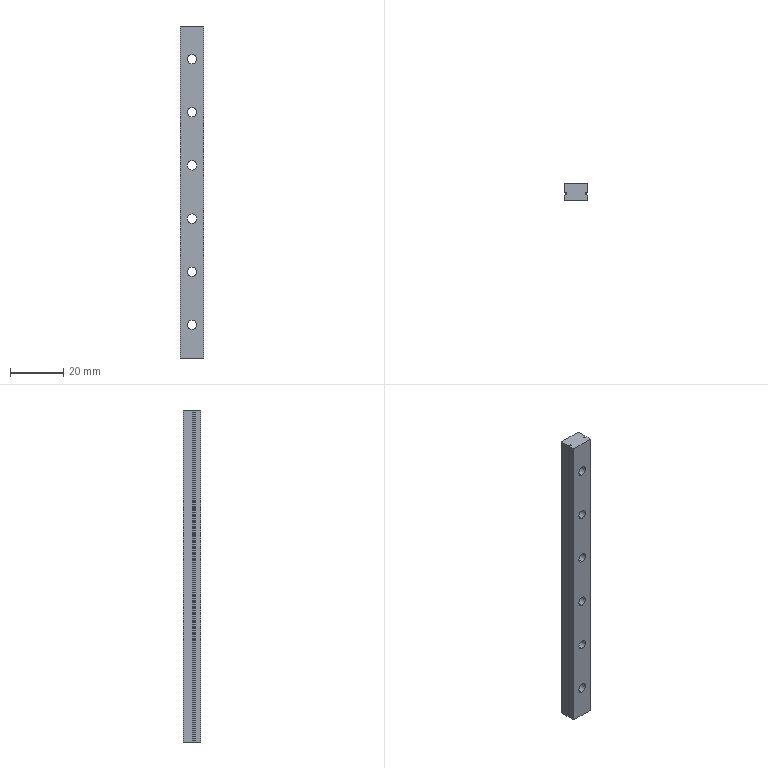Part | SolidWorks | features BaseBody 1 | 1 solid | 44 faces | box 9 x 6.5 x 125 mm | volume 6242 mm3 | cylinder 24 | plane 20 | commonest cylinder face diameters 3.5 x12 6.5 x12
STEP:
#1=CARTESIAN_POINT('',(0.,-3.25,249.25));
#2=VERTEX_POINT('',#1);
#3=CARTESIAN_POINT('',(0.,-3.25,245.75));
#4=VERTEX_POINT('',#3);
#5=CARTESIAN_POINT('',(0.,-3.25,247.5));
#6=DIRECTION('',(0.,-1.,0.));
#7=DIRECTION('',(0.,0.,1.));
#8=AXIS2_PLACEMENT_3D('',#5,#6,#7);
#9=CIRCLE('',#8,1.75);
#10=EDGE_CURVE('',#2,#4,#9,.T.);
#11=ORIENTED_EDGE('',*,*,#10,.T.);
#12=CARTESIAN_POINT('',(0.,-0.25,245.75));
#13=VERTEX_POINT('',#12);
#14=CARTESIAN_POINT('',(0.,-3.25,245.75));
#15=DIRECTION('',(0.,1.,0.));
#16=VECTOR('',#15,1000.);
#17=LINE('',#14,#16);
#18=EDGE_CURVE('',#4,#13,#17,.T.);
#19=ORIENTED_EDGE('',*,*,#18,.T.);
#20=CARTESIAN_POINT('',(0.,-0.25,249.25));
#21=VERTEX_POINT('',#20);
#22=CARTESIAN_POINT('',(0.,-0.25,247.5));
#23=DIRECTION('',(0.,-1.,0.));
#24=DIRECTION('',(0.,0.,1.));
#25=AXIS2_PLACEMENT_3D('',#22,#23,#24);
#26=CIRCLE('',#25,1.75);
#27=EDGE_CURVE('',#21,#13,#26,.T.);
#28=ORIENTED_EDGE('',*,*,#27,.F.);
#29=CARTESIAN_POINT('',(0.,-3.25,249.25));
#30=DIRECTION('',(0.,1.,0.));
#31=VECTOR('',#30,1000.);
#32=LINE('',#29,#31);
#33=EDGE_CURVE('',#2,#21,#32,.T.);
#34=ORIENTED_EDGE('',*,*,#33,.F.);
#35=EDGE_LOOP('',(#11,#19,#28,#34));
#36=FACE_OUTER_BOUND('',#35,.T.);
#37=CARTESIAN_POINT('',(0.,-3.25,247.5));
#38=DIRECTION('',(0.,1.,0.));
#39=DIRECTION('',(0.,0.,1.));
#40=AXIS2_PLACEMENT_3D('',#37,#38,#39);
#41=CYLINDRICAL_SURFACE('',#40,1.75);
#42=ADVANCED_FACE('',(#36),#41,.F.);
#43=CARTESIAN_POINT('',(0.,-3.25,229.25));
#44=VERTEX_POINT('',#43);
#45=CARTESIAN_POINT('',(0.,-3.25,225.75));
#46=VERTEX_POINT('',#45);
#47=CARTESIAN_POINT('',(0.,-3.25,227.5));
#48=DIRECTION('',(0.,-1.,0.));
#49=DIRECTION('',(0.,0.,1.));
#50=AXIS2_PLACEMENT_3D('',#47,#48,#49);
#51=CIRCLE('',#50,1.75);
#52=EDGE_CURVE('',#44,#46,#51,.T.);
#53=ORIENTED_EDGE('',*,*,#52,.T.);
#54=CARTESIAN_POINT('',(0.,-0.25,225.75));
#55=VERTEX_POINT('',#54);
#56=CARTESIAN_POINT('',(0.,-3.25,225.75));
#57=DIRECTION('',(0.,1.,0.));
#58=VECTOR('',#57,1000.);
#59=LINE('',#56,#58);
#60=EDGE_CURVE('',#46,#55,#59,.T.);
#61=ORIENTED_EDGE('',*,*,#60,.T.);
#62=CARTESIAN_POINT('',(0.,-0.25,229.25));
#63=VERTEX_POINT('',#62);
#64=CARTESIAN_POINT('',(0.,-0.25,227.5));
#65=DIRECTION('',(0.,-1.,0.));
#66=DIRECTION('',(0.,0.,1.));
#67=AXIS2_PLACEMENT_3D('',#64,#65,#66);
#68=CIRCLE('',#67,1.75);
#69=EDGE_CURVE('',#63,#55,#68,.T.);
#70=ORIENTED_EDGE('',*,*,#69,.F.);
#71=CARTESIAN_POINT('',(0.,-3.25,229.25));
#72=DIRECTION('',(0.,1.,0.));
#73=VECTOR('',#72,1000.);
#74=LINE('',#71,#73);
#75=EDGE_CURVE('',#44,#63,#74,.T.);
#76=ORIENTED_EDGE('',*,*,#75,.F.);
#77=EDGE_LOOP('',(#53,#61,#70,#76));
#78=FACE_OUTER_BOUND('',#77,.T.);
#79=CARTESIAN_POINT('',(0.,-3.25,227.5));
#80=DIRECTION('',(0.,1.,0.));
#81=DIRECTION('',(0.,0.,1.));
#82=AXIS2_PLACEMENT_3D('',#79,#80,#81);
#83=CYLINDRICAL_SURFACE('',#82,1.75);
#84=ADVANCED_FACE('',(#78),#83,.F.);
#85=CARTESIAN_POINT('',(0.,-3.25,209.25));
#86=VERTEX_POINT('',#85);
#87=CARTESIAN_POINT('',(0.,-3.25,205.75));
#88=VERTEX_POINT('',#87);
#89=CARTESIAN_POINT('',(0.,-3.25,207.5));
#90=DIRECTION('',(0.,-1.,0.));
#91=DIRECTION('',(0.,0.,1.));
#92=AXIS2_PLACEMENT_3D('',#89,#90,#91);
#93=CIRCLE('',#92,1.75);
#94=EDGE_CURVE('',#86,#88,#93,.T.);
#95=ORIENTED_EDGE('',*,*,#94,.T.);
#96=CARTESIAN_POINT('',(0.,-0.25,205.75));
#97=VERTEX_POINT('',#96);
#98=CARTESIAN_POINT('',(0.,-3.25,205.75));
#99=DIRECTION('',(0.,1.,0.));
#100=VECTOR('',#99,1000.);
#101=LINE('',#98,#100);
#102=EDGE_CURVE('',#88,#97,#101,.T.);
#103=ORIENTED_EDGE('',*,*,#102,.T.);
#104=CARTESIAN_POINT('',(0.,-0.25,209.25));
#105=VERTEX_POINT('',#104);
#106=CARTESIAN_POINT('',(0.,-0.25,207.5));
#107=DIRECTION('',(0.,-1.,0.));
#108=DIRECTION('',(0.,0.,1.));
#109=AXIS2_PLACEMENT_3D('',#106,#107,#108);
#110=CIRCLE('',#109,1.75);
#111=EDGE_CURVE('',#105,#97,#110,.T.);
#112=ORIENTED_EDGE('',*,*,#111,.F.);
#113=CARTESIAN_POINT('',(0.,-3.25,209.25));
#114=DIRECTION('',(0.,1.,0.));
#115=VECTOR('',#114,1000.);
#116=LINE('',#113,#115);
#117=EDGE_CURVE('',#86,#105,#116,.T.);
#118=ORIENTED_EDGE('',*,*,#117,.F.);
#119=EDGE_LOOP('',(#95,#103,#112,#118));
#120=FACE_OUTER_BOUND('',#119,.T.);
#121=CARTESIAN_POINT('',(0.,-3.25,207.5));
#122=DIRECTION('',(0.,1.,0.));
#123=DIRECTION('',(0.,0.,1.));
#124=AXIS2_PLACEMENT_3D('',#121,#122,#123);
#125=CYLINDRICAL_SURFACE('',#124,1.75);
#126=ADVANCED_FACE('',(#120),#125,.F.);
#127=CARTESIAN_POINT('',(0.,-3.25,189.25));
#128=VERTEX_POINT('',#127);
#129=CARTESIAN_POINT('',(0.,-3.25,185.75));
#130=VERTEX_POINT('',#129);
#131=CARTESIAN_POINT('',(0.,-3.25,187.5));
#132=DIRECTION('',(0.,-1.,0.));
#133=DIRECTION('',(0.,0.,1.));
#134=AXIS2_PLACEMENT_3D('',#131,#132,#133);
#135=CIRCLE('',#134,1.75);
#136=EDGE_CURVE('',#128,#130,#135,.T.);
#137=ORIENTED_EDGE('',*,*,#136,.T.);
#138=CARTESIAN_POINT('',(0.,-0.25,185.75));
#139=VERTEX_POINT('',#138);
#140=CARTESIAN_POINT('',(0.,-3.25,185.75));
#141=DIRECTION('',(0.,1.,0.));
#142=VECTOR('',#141,1000.);
#143=LINE('',#140,#142);
#144=EDGE_CURVE('',#130,#139,#143,.T.);
#145=ORIENTED_EDGE('',*,*,#144,.T.);
#146=CARTESIAN_POINT('',(0.,-0.25,189.25));
#147=VERTEX_POINT('',#146);
#148=CARTESIAN_POINT('',(0.,-0.25,187.5));
#149=DIRECTION('',(0.,-1.,0.));
#150=DIRECTION('',(0.,0.,1.));
#151=AXIS2_PLACEMENT_3D('',#148,#149,#150);
#152=CIRCLE('',#151,1.75);
#153=EDGE_CURVE('',#147,#139,#152,.T.);
#154=ORIENTED_EDGE('',*,*,#153,.F.);
#155=CARTESIAN_POINT('',(0.,-3.25,189.25));
#156=DIRECTION('',(0.,1.,0.));
#157=VECTOR('',#156,1000.);
#158=LINE('',#155,#157);
#159=EDGE_CURVE('',#128,#147,#158,.T.);
#160=ORIENTED_EDGE('',*,*,#159,.F.);
#161=EDGE_LOOP('',(#137,#145,#154,#160));
#162=FACE_OUTER_BOUND('',#161,.T.);
#163=CARTESIAN_POINT('',(0.,-3.25,187.5));
#164=DIRECTION('',(0.,1.,0.));
#165=DIRECTION('',(0.,0.,1.));
#166=AXIS2_PLACEMENT_3D('',#163,#164,#165);
#167=CYLINDRICAL_SURFACE('',#166,1.75);
#168=ADVANCED_FACE('',(#162),#167,.F.);
#169=CARTESIAN_POINT('',(0.,-3.25,169.25));
#170=VERTEX_POINT('',#169);
#171=CARTESIAN_POINT('',(0.,-3.25,165.75));
#172=VERTEX_POINT('',#171);
#173=CARTESIAN_POINT('',(0.,-3.25,167.5));
#174=DIRECTION('',(0.,-1.,0.));
#175=DIRECTION('',(0.,0.,1.));
#176=AXIS2_PLACEMENT_3D('',#173,#174,#175);
#177=CIRCLE('',#176,1.75);
#178=EDGE_CURVE('',#170,#172,#177,.T.);
#179=ORIENTED_EDGE('',*,*,#178,.T.);
#180=CARTESIAN_POINT('',(0.,-0.25,165.75));
#181=VERTEX_POINT('',#180);
#182=CARTESIAN_POINT('',(0.,-3.25,165.75));
#183=DIRECTION('',(0.,1.,0.));
#184=VECTOR('',#183,1000.);
#185=LINE('',#182,#184);
#186=EDGE_CURVE('',#172,#181,#185,.T.);
#187=ORIENTED_EDGE('',*,*,#186,.T.);
#188=CARTESIAN_POINT('',(0.,-0.25,169.25));
#189=VERTEX_POINT('',#188);
#190=CARTESIAN_POINT('',(0.,-0.25,167.5));
#191=DIRECTION('',(0.,-1.,0.));
#192=DIRECTION('',(0.,0.,1.));
#193=AXIS2_PLACEMENT_3D('',#190,#191,#192);
#194=CIRCLE('',#193,1.75);
#195=EDGE_CURVE('',#189,#181,#194,.T.);
#196=ORIENTED_EDGE('',*,*,#195,.F.);
#197=CARTESIAN_POINT('',(0.,-3.25,169.25));
#198=DIRECTION('',(0.,1.,0.));
#199=VECTOR('',#198,1000.);
#200=LINE('',#197,#199);
#201=EDGE_CURVE('',#170,#189,#200,.T.);
#202=ORIENTED_EDGE('',*,*,#201,.F.);
#203=EDGE_LOOP('',(#179,#187,#196,#202));
#204=FACE_OUTER_BOUND('',#203,.T.);
#205=CARTESIAN_POINT('',(0.,-3.25,167.5));
#206=DIRECTION('',(0.,1.,0.));
#207=DIRECTION('',(0.,0.,1.));
#208=AXIS2_PLACEMENT_3D('',#205,#206,#207);
#209=CYLINDRICAL_SURFACE('',#208,1.75);
#210=ADVANCED_FACE('',(#204),#209,.F.);
#211=CARTESIAN_POINT('',(0.,-3.25,149.25));
#212=VERTEX_POINT('',#211);
#213=CARTESIAN_POINT('',(0.,-3.25,145.75));
#214=VERTEX_POINT('',#213);
#215=CARTESIAN_POINT('',(0.,-3.25,147.5));
#216=DIRECTION('',(0.,-1.,0.));
#217=DIRECTION('',(0.,0.,1.));
#218=AXIS2_PLACEMENT_3D('',#215,#216,#217);
#219=CIRCLE('',#218,1.75);
#220=EDGE_CURVE('',#212,#214,#219,.T.);
#221=ORIENTED_EDGE('',*,*,#220,.T.);
#222=CARTESIAN_POINT('',(0.,-0.25,145.75));
#223=VERTEX_POINT('',#222);
#224=CARTESIAN_POINT('',(0.,-3.25,145.75));
#225=DIRECTION('',(0.,1.,0.));
#226=VECTOR('',#225,1000.);
#227=LINE('',#224,#226);
#228=EDGE_CURVE('',#214,#223,#227,.T.);
#229=ORIENTED_EDGE('',*,*,#228,.T.);
#230=CARTESIAN_POINT('',(0.,-0.25,149.25));
#231=VERTEX_POINT('',#230);
#232=CARTESIAN_POINT('',(0.,-0.25,147.5));
#233=DIRECTION('',(0.,-1.,0.));
#234=DIRECTION('',(0.,0.,1.));
#235=AXIS2_PLACEMENT_3D('',#232,#233,#234);
#236=CIRCLE('',#235,1.75);
#237=EDGE_CURVE('',#231,#223,#236,.T.);
#238=ORIENTED_EDGE('',*,*,#237,.F.);
#239=CARTESIAN_POINT('',(0.,-3.25,149.25));
#240=DIRECTION('',(0.,1.,0.));
#241=VECTOR('',#240,1000.);
#242=LINE('',#239,#241);
#243=EDGE_CURVE('',#212,#231,#242,.T.);
#244=ORIENTED_EDGE('',*,*,#243,.F.);
#245=EDGE_LOOP('',(#221,#229,#238,#244));
#246=FACE_OUTER_BOUND('',#245,.T.);
#247=CARTESIAN_POINT('',(0.,-3.25,147.5));
#248=DIRECTION('',(0.,1.,0.));
#249=DIRECTION('',(0.,0.,1.));
#250=AXIS2_PLACEMENT_3D('',#247,#248,#249);
#251=CYLINDRICAL_SURFACE('',#250,1.75);
#252=ADVANCED_FACE('',(#246),#251,.F.);
#253=CARTESIAN_POINT('',(0.,-0.25,244.25));
#254=VERTEX_POINT('',#253);
#255=CARTESIAN_POINT('',(0.,-0.25,250.75));
#256=VERTEX_POINT('',#255);
#257=CARTESIAN_POINT('',(0.,-0.25,247.5));
#258=DIRECTION('',(0.,1.,0.));
#259=DIRECTION('',(0.,0.,1.));
#260=AXIS2_PLACEMENT_3D('',#257,#258,#259);
#261=CIRCLE('',#260,3.25);
#262=EDGE_CURVE('',#254,#256,#261,.T.);
#263=ORIENTED_EDGE('',*,*,#262,.F.);
#264=CARTESIAN_POINT('',(0.,3.25,244.25));
#265=VERTEX_POINT('',#264);
#266=CARTESIAN_POINT('',(0.,-0.25,244.25));
#267=DIRECTION('',(0.,1.,0.));
#268=VECTOR('',#267,1000.);
#269=LINE('',#266,#268);
#270=EDGE_CURVE('',#254,#265,#269,.T.);
#271=ORIENTED_EDGE('',*,*,#270,.T.);
#272=CARTESIAN_POINT('',(0.,3.25,250.75));
#273=VERTEX_POINT('',#272);
#274=CARTESIAN_POINT('',(0.,3.25,247.5));
#275=DIRECTION('',(0.,1.,0.));
#276=DIRECTION('',(0.,0.,1.));
#277=AXIS2_PLACEMENT_3D('',#274,#275,#276);
#278=CIRCLE('',#277,3.25);
#279=EDGE_CURVE('',#265,#273,#278,.T.);
#280=ORIENTED_EDGE('',*,*,#279,.T.);
#281=CARTESIAN_POINT('',(0.,-0.25,250.75));
#282=DIRECTION('',(0.,1.,0.));
#283=VECTOR('',#282,1000.);
#284=LINE('',#281,#283);
#285=EDGE_CURVE('',#256,#273,#284,.T.);
#286=ORIENTED_EDGE('',*,*,#285,.F.);
#287=EDGE_LOOP('',(#263,#271,#280,#286));
#288=FACE_OUTER_BOUND('',#287,.T.);
#289=CARTESIAN_POINT('',(0.,-0.25,247.5));
#290=DIRECTION('',(0.,1.,0.));
#291=DIRECTION('',(0.,0.,1.));
#292=AXIS2_PLACEMENT_3D('',#289,#290,#291);
#293=CYLINDRICAL_SURFACE('',#292,3.25);
#294=ADVANCED_FACE('',(#288),#293,.F.);
#295=CARTESIAN_POINT('',(0.,-0.25,224.25));
#296=VERTEX_POINT('',#295);
#297=CARTESIAN_POINT('',(0.,-0.25,230.75));
#298=VERTEX_POINT('',#297);
#299=CARTESIAN_POINT('',(0.,-0.25,227.5));
#300=DIRECTION('',(0.,1.,0.));
#301=DIRECTION('',(0.,0.,1.));
#302=AXIS2_PLACEMENT_3D('',#299,#300,#301);
#303=CIRCLE('',#302,3.25);
#304=EDGE_CURVE('',#296,#298,#303,.T.);
#305=ORIENTED_EDGE('',*,*,#304,.F.);
#306=CARTESIAN_POINT('',(0.,3.25,224.25));
#307=VERTEX_POINT('',#306);
#308=CARTESIAN_POINT('',(0.,-0.25,224.25));
#309=DIRECTION('',(0.,1.,0.));
#310=VECTOR('',#309,1000.);
#311=LINE('',#308,#310);
#312=EDGE_CURVE('',#296,#307,#311,.T.);
#313=ORIENTED_EDGE('',*,*,#312,.T.);
#314=CARTESIAN_POINT('',(0.,3.25,230.75));
#315=VERTEX_POINT('',#314);
#316=CARTESIAN_POINT('',(0.,3.25,227.5));
#317=DIRECTION('',(0.,1.,0.));
#318=DIRECTION('',(0.,0.,1.));
#319=AXIS2_PLACEMENT_3D('',#316,#317,#318);
#320=CIRCLE('',#319,3.25);
#321=EDGE_CURVE('',#307,#315,#320,.T.);
#322=ORIENTED_EDGE('',*,*,#321,.T.);
#323=CARTESIAN_POINT('',(0.,-0.25,230.75));
#324=DIRECTION('',(0.,1.,0.));
#325=VECTOR('',#324,1000.);
#326=LINE('',#323,#325);
#327=EDGE_CURVE('',#298,#315,#326,.T.);
#328=ORIENTED_EDGE('',*,*,#327,.F.);
#329=EDGE_LOOP('',(#305,#313,#322,#328));
#330=FACE_OUTER_BOUND('',#329,.T.);
#331=CARTESIAN_POINT('',(0.,-0.25,227.5));
#332=DIRECTION('',(0.,1.,0.));
#333=DIRECTION('',(0.,0.,1.));
#334=AXIS2_PLACEMENT_3D('',#331,#332,#333);
#335=CYLINDRICAL_SURFACE('',#334,3.25);
#336=ADVANCED_FACE('',(#330),#335,.F.);
#337=CARTESIAN_POINT('',(0.,-0.25,204.25));
#338=VERTEX_POINT('',#337);
#339=CARTESIAN_POINT('',(0.,-0.25,210.75));
#340=VERTEX_POINT('',#339);
#341=CARTESIAN_POINT('',(0.,-0.25,207.5));
#342=DIRECTION('',(0.,1.,0.));
#343=DIRECTION('',(0.,0.,1.));
#344=AXIS2_PLACEMENT_3D('',#341,#342,#343);
#345=CIRCLE('',#344,3.25);
#346=EDGE_CURVE('',#338,#340,#345,.T.);
#347=ORIENTED_EDGE('',*,*,#346,.F.);
#348=CARTESIAN_POINT('',(0.,3.25,204.25));
#349=VERTEX_POINT('',#348);
#350=CARTESIAN_POINT('',(0.,-0.25,204.25));
#351=DIRECTION('',(0.,1.,0.));
#352=VECTOR('',#351,1000.);
#353=LINE('',#350,#352);
#354=EDGE_CURVE('',#338,#349,#353,.T.);
#355=ORIENTED_EDGE('',*,*,#354,.T.);
#356=CARTESIAN_POINT('',(0.,3.25,210.75));
#357=VERTEX_POINT('',#356);
#358=CARTESIAN_POINT('',(0.,3.25,207.5));
#359=DIRECTION('',(0.,1.,0.));
#360=DIRECTION('',(0.,0.,1.));
#361=AXIS2_PLACEMENT_3D('',#358,#359,#360);
#362=CIRCLE('',#361,3.25);
#363=EDGE_CURVE('',#349,#357,#362,.T.);
#364=ORIENTED_EDGE('',*,*,#363,.T.);
#365=CARTESIAN_POINT('',(0.,-0.25,210.75));
#366=DIRECTION('',(0.,1.,0.));
#367=VECTOR('',#366,1000.);
#368=LINE('',#365,#367);
#369=EDGE_CURVE('',#340,#357,#368,.T.);
#370=ORIENTED_EDGE('',*,*,#369,.F.);
#371=EDGE_LOOP('',(#347,#355,#364,#370));
#372=FACE_OUTER_BOUND('',#371,.T.);
#373=CARTESIAN_POINT('',(0.,-0.25,207.5));
#374=DIRECTION('',(0.,1.,0.));
#375=DIRECTION('',(0.,0.,1.));
#376=AXIS2_PLACEMENT_3D('',#373,#374,#375);
#377=CYLINDRICAL_SURFACE('',#376,3.25);
#378=ADVANCED_FACE('',(#372),#377,.F.);
#379=CARTESIAN_POINT('',(0.,-0.25,184.25));
#380=VERTEX_POINT('',#379);
#381=CARTESIAN_POINT('',(0.,-0.25,190.75));
#382=VERTEX_POINT('',#381);
#383=CARTESIAN_POINT('',(0.,-0.25,187.5));
#384=DIRECTION('',(0.,1.,0.));
#385=DIRECTION('',(0.,0.,1.));
#386=AXIS2_PLACEMENT_3D('',#383,#384,#385);
#387=CIRCLE('',#386,3.25);
#388=EDGE_CURVE('',#380,#382,#387,.T.);
#389=ORIENTED_EDGE('',*,*,#388,.F.);
#390=CARTESIAN_POINT('',(0.,3.25,184.25));
#391=VERTEX_POINT('',#390);
#392=CARTESIAN_POINT('',(0.,-0.25,184.25));
#393=DIRECTION('',(0.,1.,0.));
#394=VECTOR('',#393,1000.);
#395=LINE('',#392,#394);
#396=EDGE_CURVE('',#380,#391,#395,.T.);
#397=ORIENTED_EDGE('',*,*,#396,.T.);
#398=CARTESIAN_POINT('',(0.,3.25,190.75));
#399=VERTEX_POINT('',#398);
#400=CARTESIAN_POINT('',(0.,3.25,187.5));
#401=DIRECTION('',(0.,1.,0.));
#402=DIRECTION('',(0.,0.,1.));
#403=AXIS2_PLACEMENT_3D('',#400,#401,#402);
#404=CIRCLE('',#403,3.25);
#405=EDGE_CURVE('',#391,#399,#404,.T.);
#406=ORIENTED_EDGE('',*,*,#405,.T.);
#407=CARTESIAN_POINT('',(0.,-0.25,190.75));
#408=DIRECTION('',(0.,1.,0.));
#409=VECTOR('',#408,1000.);
#410=LINE('',#407,#409);
#411=EDGE_CURVE('',#382,#399,#410,.T.);
#412=ORIENTED_EDGE('',*,*,#411,.F.);
#413=EDGE_LOOP('',(#389,#397,#406,#412));
#414=FACE_OUTER_BOUND('',#413,.T.);
#415=CARTESIAN_POINT('',(0.,-0.25,187.5));
#416=DIRECTION('',(0.,1.,0.));
#417=DIRECTION('',(0.,0.,1.));
#418=AXIS2_PLACEMENT_3D('',#415,#416,#417);
#419=CYLINDRICAL_SURFACE('',#418,3.25);
#420=ADVANCED_FACE('',(#414),#419,.F.);
#421=CARTESIAN_POINT('',(0.,-0.25,164.25));
#422=VERTEX_POINT('',#421);
#423=CARTESIAN_POINT('',(0.,-0.25,170.75));
#424=VERTEX_POINT('',#423);
#425=CARTESIAN_POINT('',(0.,-0.25,167.5));
#426=DIRECTION('',(0.,1.,0.));
#427=DIRECTION('',(0.,0.,1.));
#428=AXIS2_PLACEMENT_3D('',#425,#426,#427);
#429=CIRCLE('',#428,3.25);
#430=EDGE_CURVE('',#422,#424,#429,.T.);
#431=ORIENTED_EDGE('',*,*,#430,.F.);
#432=CARTESIAN_POINT('',(0.,3.25,164.25));
#433=VERTEX_POINT('',#432);
#434=CARTESIAN_POINT('',(0.,-0.25,164.25));
#435=DIRECTION('',(0.,1.,0.));
#436=VECTOR('',#435,1000.);
#437=LINE('',#434,#436);
#438=EDGE_CURVE('',#422,#433,#437,.T.);
#439=ORIENTED_EDGE('',*,*,#438,.T.);
#440=CARTESIAN_POINT('',(0.,3.25,170.75));
#441=VERTEX_POINT('',#440);
#442=CARTESIAN_POINT('',(0.,3.25,167.5));
#443=DIRECTION('',(0.,1.,0.));
#444=DIRECTION('',(0.,0.,1.));
#445=AXIS2_PLACEMENT_3D('',#442,#443,#444);
#446=CIRCLE('',#445,3.25);
#447=EDGE_CURVE('',#433,#441,#446,.T.);
#448=ORIENTED_EDGE('',*,*,#447,.T.);
#449=CARTESIAN_POINT('',(0.,-0.25,170.75));
#450=DIRECTION('',(0.,1.,0.));
#451=VECTOR('',#450,1000.);
#452=LINE('',#449,#451);
#453=EDGE_CURVE('',#424,#441,#452,.T.);
#454=ORIENTED_EDGE('',*,*,#453,.F.);
#455=EDGE_LOOP('',(#431,#439,#448,#454));
#456=FACE_OUTER_BOUND('',#455,.T.);
#457=CARTESIAN_POINT('',(0.,-0.25,167.5));
#458=DIRECTION('',(0.,1.,0.));
#459=DIRECTION('',(0.,0.,1.));
#460=AXIS2_PLACEMENT_3D('',#457,#458,#459);
#461=CYLINDRICAL_SURFACE('',#460,3.25);
#462=ADVANCED_FACE('',(#456),#461,.F.);
#463=CARTESIAN_POINT('',(0.,-0.25,144.25));
#464=VERTEX_POINT('',#463);
#465=CARTESIAN_POINT('',(0.,-0.25,150.75));
#466=VERTEX_POINT('',#465);
#467=CARTESIAN_POINT('',(0.,-0.25,147.5));
#468=DIRECTION('',(0.,1.,0.));
#469=DIRECTION('',(0.,0.,1.));
#470=AXIS2_PLACEMENT_3D('',#467,#468,#469);
#471=CIRCLE('',#470,3.25);
#472=EDGE_CURVE('',#464,#466,#471,.T.);
#473=ORIENTED_EDGE('',*,*,#472,.F.);
#474=CARTESIAN_POINT('',(0.,3.25,144.25));
#475=VERTEX_POINT('',#474);
#476=CARTESIAN_POINT('',(0.,-0.25,144.25));
#477=DIRECTION('',(0.,1.,0.));
#478=VECTOR('',#477,1000.);
#479=LINE('',#476,#478);
#480=EDGE_CURVE('',#464,#475,#479,.T.);
#481=ORIENTED_EDGE('',*,*,#480,.T.);
#482=CARTESIAN_POINT('',(0.,3.25,150.75));
#483=VERTEX_POINT('',#482);
#484=CARTESIAN_POINT('',(0.,3.25,147.5));
#485=DIRECTION('',(0.,1.,0.));
#486=DIRECTION('',(0.,0.,1.));
#487=AXIS2_PLACEMENT_3D('',#484,#485,#486);
#488=CIRCLE('',#487,3.25);
#489=EDGE_CURVE('',#475,#483,#488,.T.);
#490=ORIENTED_EDGE('',*,*,#489,.T.);
#491=CARTESIAN_POINT('',(0.,-0.25,150.75));
#492=DIRECTION('',(0.,1.,0.));
#493=VECTOR('',#492,1000.);
#494=LINE('',#491,#493);
#495=EDGE_CURVE('',#466,#483,#494,.T.);
#496=ORIENTED_EDGE('',*,*,#495,.F.);
#497=EDGE_LOOP('',(#473,#481,#490,#496));
#498=FACE_OUTER_BOUND('',#497,.T.);
#499=CARTESIAN_POINT('',(0.,-0.25,147.5));
#500=DIRECTION('',(0.,1.,0.));
#501=DIRECTION('',(0.,0.,1.));
#502=AXIS2_PLACEMENT_3D('',#499,#500,#501);
#503=CYLINDRICAL_SURFACE('',#502,3.25);
#504=ADVANCED_FACE('',(#498),#503,.F.);
#505=CARTESIAN_POINT('',(4.5,-3.25,135.));
#506=VERTEX_POINT('',#505);
#507=CARTESIAN_POINT('',(-4.5,-3.25,135.));
#508=VERTEX_POINT('',#507);
#509=CARTESIAN_POINT('',(-4.5,-3.25,135.));
#510=DIRECTION('',(-1.,0.,0.));
#511=VECTOR('',#510,1000.);
#512=LINE('',#509,#511);
#513=EDGE_CURVE('',#506,#508,#512,.T.);
#514=ORIENTED_EDGE('',*,*,#513,.F.);
#515=CARTESIAN_POINT('',(4.5,-3.25,260.));
#516=VERTEX_POINT('',#515);
#517=CARTESIAN_POINT('',(4.5,-3.25,260.));
#518=DIRECTION('',(0.,0.,-1.));
#519=VECTOR('',#518,1000.);
#520=LINE('',#517,#519);
#521=EDGE_CURVE('',#516,#506,#520,.T.);
#522=ORIENTED_EDGE('',*,*,#521,.F.);
#523=CARTESIAN_POINT('',(-4.5,-3.25,260.));
#524=VERTEX_POINT('',#523);
#525=CARTESIAN_POINT('',(-4.5,-3.25,260.));
#526=DIRECTION('',(1.,0.,0.));
#527=VECTOR('',#526,1000.);
#528=LINE('',#525,#527);
#529=EDGE_CURVE('',#524,#516,#528,.T.);
#530=ORIENTED_EDGE('',*,*,#529,.F.);
#531=CARTESIAN_POINT('',(-4.5,-3.25,260.));
#532=DIRECTION('',(0.,0.,1.));
#533=VECTOR('',#532,1000.);
#534=LINE('',#531,#533);
#535=EDGE_CURVE('',#508,#524,#534,.T.);
#536=ORIENTED_EDGE('',*,*,#535,.F.);
#537=EDGE_LOOP('',(#514,#522,#530,#536));
#538=FACE_OUTER_BOUND('',#537,.T.);
#539=ORIENTED_EDGE('',*,*,#10,.F.);
#540=CARTESIAN_POINT('',(0.,-3.25,247.5));
#541=DIRECTION('',(0.,-1.,0.));
#542=DIRECTION('',(0.,0.,1.));
#543=AXIS2_PLACEMENT_3D('',#540,#541,#542);
#544=CIRCLE('',#543,1.75);
#545=EDGE_CURVE('',#4,#2,#544,.T.);
#546=ORIENTED_EDGE('',*,*,#545,.F.);
#547=EDGE_LOOP('',(#539,#546));
#548=FACE_BOUND('',#547,.T.);
#549=ORIENTED_EDGE('',*,*,#52,.F.);
#550=CARTESIAN_POINT('',(0.,-3.25,227.5));
#551=DIRECTION('',(0.,-1.,0.));
#552=DIRECTION('',(0.,0.,1.));
#553=AXIS2_PLACEMENT_3D('',#550,#551,#552);
#554=CIRCLE('',#553,1.75);
#555=EDGE_CURVE('',#46,#44,#554,.T.);
#556=ORIENTED_EDGE('',*,*,#555,.F.);
#557=EDGE_LOOP('',(#549,#556));
#558=FACE_BOUND('',#557,.T.);
#559=ORIENTED_EDGE('',*,*,#94,.F.);
#560=CARTESIAN_POINT('',(0.,-3.25,207.5));
#561=DIRECTION('',(0.,-1.,0.));
#562=DIRECTION('',(0.,0.,1.));
#563=AXIS2_PLACEMENT_3D('',#560,#561,#562);
#564=CIRCLE('',#563,1.75);
#565=EDGE_CURVE('',#88,#86,#564,.T.);
#566=ORIENTED_EDGE('',*,*,#565,.F.);
#567=EDGE_LOOP('',(#559,#566));
#568=FACE_BOUND('',#567,.T.);
#569=ORIENTED_EDGE('',*,*,#136,.F.);
#570=CARTESIAN_POINT('',(0.,-3.25,187.5));
#571=DIRECTION('',(0.,-1.,0.));
#572=DIRECTION('',(0.,0.,1.));
#573=AXIS2_PLACEMENT_3D('',#570,#571,#572);
#574=CIRCLE('',#573,1.75);
#575=EDGE_CURVE('',#130,#128,#574,.T.);
#576=ORIENTED_EDGE('',*,*,#575,.F.);
#577=EDGE_LOOP('',(#569,#576));
#578=FACE_BOUND('',#577,.T.);
#579=ORIENTED_EDGE('',*,*,#178,.F.);
#580=CARTESIAN_POINT('',(0.,-3.25,167.5));
#581=DIRECTION('',(0.,-1.,0.));
#582=DIRECTION('',(0.,0.,1.));
#583=AXIS2_PLACEMENT_3D('',#580,#581,#582);
#584=CIRCLE('',#583,1.75);
#585=EDGE_CURVE('',#172,#170,#584,.T.);
#586=ORIENTED_EDGE('',*,*,#585,.F.);
#587=EDGE_LOOP('',(#579,#586));
#588=FACE_BOUND('',#587,.T.);
#589=ORIENTED_EDGE('',*,*,#220,.F.);
#590=CARTESIAN_POINT('',(0.,-3.25,147.5));
#591=DIRECTION('',(0.,-1.,0.));
#592=DIRECTION('',(0.,0.,1.));
#593=AXIS2_PLACEMENT_3D('',#590,#591,#592);
#594=CIRCLE('',#593,1.75);
#595=EDGE_CURVE('',#214,#212,#594,.T.);
#596=ORIENTED_EDGE('',*,*,#595,.F.);
#597=EDGE_LOOP('',(#589,#596));
#598=FACE_BOUND('',#597,.T.);
#599=CARTESIAN_POINT('',(-4.5,-3.25,260.));
#600=DIRECTION('',(0.,1.,0.));
#601=DIRECTION('',(0.,0.,1.));
#602=AXIS2_PLACEMENT_3D('',#599,#600,#601);
#603=PLANE('',#602);
#604=ADVANCED_FACE('',(#538,#548,#558,#568,#578,#588,#598),#603,.F.);
#605=CARTESIAN_POINT('',(-4.5,-1.25,135.));
#606=VERTEX_POINT('',#605);
#607=CARTESIAN_POINT('',(-4.5,3.25,135.));
#608=DIRECTION('',(0.,1.,0.));
#609=VECTOR('',#608,1000.);
#610=LINE('',#607,#609);
#611=EDGE_CURVE('',#508,#606,#610,.T.);
#612=ORIENTED_EDGE('',*,*,#611,.F.);
#613=ORIENTED_EDGE('',*,*,#535,.T.);
#614=CARTESIAN_POINT('',(-4.5,-1.25,260.));
#615=VERTEX_POINT('',#614);
#616=CARTESIAN_POINT('',(-4.5,3.25,260.));
#617=DIRECTION('',(0.,-1.,0.));
#618=VECTOR('',#617,1000.);
#619=LINE('',#616,#618);
#620=EDGE_CURVE('',#615,#524,#619,.T.);
#621=ORIENTED_EDGE('',*,*,#620,.F.);
#622=CARTESIAN_POINT('',(-4.5,-1.25,260.));
#623=DIRECTION('',(0.,0.,1.));
#624=VECTOR('',#623,1000.);
#625=LINE('',#622,#624);
#626=EDGE_CURVE('',#606,#615,#625,.T.);
#627=ORIENTED_EDGE('',*,*,#626,.F.);
#628=EDGE_LOOP('',(#612,#613,#621,#627));
#629=FACE_OUTER_BOUND('',#628,.T.);
#630=CARTESIAN_POINT('',(-4.5,3.25,260.));
#631=DIRECTION('',(1.,0.,0.));
#632=DIRECTION('',(0.,1.,0.));
#633=AXIS2_PLACEMENT_3D('',#630,#631,#632);
#634=PLANE('',#633);
#635=ADVANCED_FACE('',(#629),#634,.F.);
#636=CARTESIAN_POINT('',(-3.5,-1.05,135.));
#637=VERTEX_POINT('',#636);
#638=CARTESIAN_POINT('',(-3.5,-1.05,135.));
#639=DIRECTION('',(-0.9806,-0.1961,0.));
#640=VECTOR('',#639,1000.);
#641=LINE('',#638,#640);
#642=EDGE_CURVE('',#637,#606,#641,.T.);
#643=ORIENTED_EDGE('',*,*,#642,.F.);
#644=CARTESIAN_POINT('',(-3.5,-0.45,135.));
#645=VERTEX_POINT('',#644);
#646=CARTESIAN_POINT('',(-3.5,-0.45,135.));
#647=DIRECTION('',(0.,1.,0.));
#648=VECTOR('',#647,1000.);
#649=LINE('',#646,#648);
#650=EDGE_CURVE('',#637,#645,#649,.T.);
#651=ORIENTED_EDGE('',*,*,#650,.T.);
#652=CARTESIAN_POINT('',(-4.5,-0.25,135.));
#653=VERTEX_POINT('',#652);
#654=CARTESIAN_POINT('',(-4.5,-0.25,135.));
#655=DIRECTION('',(-0.9806,0.1961,0.));
#656=VECTOR('',#655,1000.);
#657=LINE('',#654,#656);
#658=EDGE_CURVE('',#645,#653,#657,.T.);
#659=ORIENTED_EDGE('',*,*,#658,.T.);
#660=CARTESIAN_POINT('',(-4.5,3.25,135.));
#661=VERTEX_POINT('',#660);
#662=CARTESIAN_POINT('',(-4.5,-6.75,135.));
#663=DIRECTION('',(0.,-1.,0.));
#664=VECTOR('',#663,1000.);
#665=LINE('',#662,#664);
#666=EDGE_CURVE('',#661,#653,#665,.T.);
#667=ORIENTED_EDGE('',*,*,#666,.F.);
#668=CARTESIAN_POINT('',(4.5,3.25,135.));
#669=VERTEX_POINT('',#668);
#670=CARTESIAN_POINT('',(-4.5,3.25,135.));
#671=DIRECTION('',(-1.,0.,0.));
#672=VECTOR('',#671,1000.);
#673=LINE('',#670,#672);
#674=EDGE_CURVE('',#669,#661,#673,.T.);
#675=ORIENTED_EDGE('',*,*,#674,.F.);
#676=CARTESIAN_POINT('',(4.5,-0.25,135.));
#677=VERTEX_POINT('',#676);
#678=CARTESIAN_POINT('',(4.5,-6.75,135.));
#679=DIRECTION('',(0.,1.,0.));
#680=VECTOR('',#679,1000.);
#681=LINE('',#678,#680);
#682=EDGE_CURVE('',#677,#669,#681,.T.);
#683=ORIENTED_EDGE('',*,*,#682,.F.);
#684=CARTESIAN_POINT('',(3.5,-0.45,135.));
#685=VERTEX_POINT('',#684);
#686=CARTESIAN_POINT('',(4.5,-0.25,135.));
#687=DIRECTION('',(-0.9806,-0.1961,0.));
#688=VECTOR('',#687,1000.);
#689=LINE('',#686,#688);
#690=EDGE_CURVE('',#677,#685,#689,.T.);
#691=ORIENTED_EDGE('',*,*,#690,.T.);
#692=CARTESIAN_POINT('',(3.5,-1.05,135.));
#693=VERTEX_POINT('',#692);
#694=CARTESIAN_POINT('',(3.5,-0.45,135.));
#695=DIRECTION('',(0.,-1.,0.));
#696=VECTOR('',#695,1000.);
#697=LINE('',#694,#696);
#698=EDGE_CURVE('',#685,#693,#697,.T.);
#699=ORIENTED_EDGE('',*,*,#698,.T.);
#700=CARTESIAN_POINT('',(4.5,-1.25,135.));
#701=VERTEX_POINT('',#700);
#702=CARTESIAN_POINT('',(3.5,-1.05,135.));
#703=DIRECTION('',(0.9806,-0.1961,0.));
#704=VECTOR('',#703,1000.);
#705=LINE('',#702,#704);
#706=EDGE_CURVE('',#693,#701,#705,.T.);
#707=ORIENTED_EDGE('',*,*,#706,.T.);
#708=CARTESIAN_POINT('',(4.5,-6.75,135.));
#709=DIRECTION('',(0.,1.,0.));
#710=VECTOR('',#709,1000.);
#711=LINE('',#708,#710);
#712=EDGE_CURVE('',#506,#701,#711,.T.);
#713=ORIENTED_EDGE('',*,*,#712,.F.);
#714=ORIENTED_EDGE('',*,*,#513,.T.);
#715=ORIENTED_EDGE('',*,*,#611,.T.);
#716=EDGE_LOOP('',(#643,#651,#659,#667,#675,#683,#691,#699,#707,#713,#714,#715));
#717=FACE_OUTER_BOUND('',#716,.T.);
#718=CARTESIAN_POINT('',(-4.5,-6.75,135.));
#719=DIRECTION('',(0.,0.,1.));
#720=DIRECTION('',(1.,0.,0.));
#721=AXIS2_PLACEMENT_3D('',#718,#719,#720);
#722=PLANE('',#721);
#723=ADVANCED_FACE('',(#717),#722,.F.);
#724=ORIENTED_EDGE('',*,*,#712,.T.);
#725=CARTESIAN_POINT('',(4.5,-1.25,260.));
#726=VERTEX_POINT('',#725);
#727=CARTESIAN_POINT('',(4.5,-1.25,260.));
#728=DIRECTION('',(0.,0.,-1.));
#729=VECTOR('',#728,1000.);
#730=LINE('',#727,#729);
#731=EDGE_CURVE('',#726,#701,#730,.T.);
#732=ORIENTED_EDGE('',*,*,#731,.F.);
#733=CARTESIAN_POINT('',(4.5,3.25,260.));
#734=DIRECTION('',(0.,1.,0.));
#735=VECTOR('',#734,1000.);
#736=LINE('',#733,#735);
#737=EDGE_CURVE('',#516,#726,#736,.T.);
#738=ORIENTED_EDGE('',*,*,#737,.F.);
#739=ORIENTED_EDGE('',*,*,#521,.T.);
#740=EDGE_LOOP('',(#724,#732,#738,#739));
#741=FACE_OUTER_BOUND('',#740,.T.);
#742=CARTESIAN_POINT('',(4.5,3.25,260.));
#743=DIRECTION('',(-1.,0.,0.));
#744=DIRECTION('',(0.,0.,1.));
#745=AXIS2_PLACEMENT_3D('',#742,#743,#744);
#746=PLANE('',#745);
#747=ADVANCED_FACE('',(#741),#746,.F.);
#748=CARTESIAN_POINT('',(-4.5,-0.25,260.));
#749=VERTEX_POINT('',#748);
#750=CARTESIAN_POINT('',(-3.5,-0.45,260.));
#751=VERTEX_POINT('',#750);
#752=CARTESIAN_POINT('',(-4.5,-0.25,260.));
#753=DIRECTION('',(0.9806,-0.1961,0.));
#754=VECTOR('',#753,1000.);
#755=LINE('',#752,#754);
#756=EDGE_CURVE('',#749,#751,#755,.T.);
#757=ORIENTED_EDGE('',*,*,#756,.T.);
#758=CARTESIAN_POINT('',(-3.5,-1.05,260.));
#759=VERTEX_POINT('',#758);
#760=CARTESIAN_POINT('',(-3.5,-0.45,260.));
#761=DIRECTION('',(0.,-1.,0.));
#762=VECTOR('',#761,1000.);
#763=LINE('',#760,#762);
#764=EDGE_CURVE('',#751,#759,#763,.T.);
#765=ORIENTED_EDGE('',*,*,#764,.T.);
#766=CARTESIAN_POINT('',(-3.5,-1.05,260.));
#767=DIRECTION('',(-0.9806,-0.1961,0.));
#768=VECTOR('',#767,1000.);
#769=LINE('',#766,#768);
#770=EDGE_CURVE('',#759,#615,#769,.T.);
#771=ORIENTED_EDGE('',*,*,#770,.T.);
#772=ORIENTED_EDGE('',*,*,#620,.T.);
#773=ORIENTED_EDGE('',*,*,#529,.T.);
#774=ORIENTED_EDGE('',*,*,#737,.T.);
#775=CARTESIAN_POINT('',(3.5,-1.05,260.));
#776=VERTEX_POINT('',#775);
#777=CARTESIAN_POINT('',(4.5,-1.25,260.));
#778=DIRECTION('',(-0.9806,0.1961,0.));
#779=VECTOR('',#778,1000.);
#780=LINE('',#777,#779);
#781=EDGE_CURVE('',#726,#776,#780,.T.);
#782=ORIENTED_EDGE('',*,*,#781,.T.);
#783=CARTESIAN_POINT('',(3.5,-0.45,260.));
#784=VERTEX_POINT('',#783);
#785=CARTESIAN_POINT('',(3.5,-0.45,260.));
#786=DIRECTION('',(0.,1.,0.));
#787=VECTOR('',#786,1000.);
#788=LINE('',#785,#787);
#789=EDGE_CURVE('',#776,#784,#788,.T.);
#790=ORIENTED_EDGE('',*,*,#789,.T.);
#791=CARTESIAN_POINT('',(4.5,-0.25,260.));
#792=VERTEX_POINT('',#791);
#793=CARTESIAN_POINT('',(4.5,-0.25,260.));
#794=DIRECTION('',(0.9806,0.1961,0.));
#795=VECTOR('',#794,1000.);
#796=LINE('',#793,#795);
#797=EDGE_CURVE('',#784,#792,#796,.T.);
#798=ORIENTED_EDGE('',*,*,#797,.T.);
#799=CARTESIAN_POINT('',(4.5,3.25,260.));
#800=VERTEX_POINT('',#799);
#801=CARTESIAN_POINT('',(4.5,0.,260.));
#802=DIRECTION('',(0.,1.,0.));
#803=VECTOR('',#802,1000.);
#804=LINE('',#801,#803);
#805=EDGE_CURVE('',#792,#800,#804,.T.);
#806=ORIENTED_EDGE('',*,*,#805,.T.);
#807=CARTESIAN_POINT('',(-4.5,3.25,260.));
#808=VERTEX_POINT('',#807);
#809=CARTESIAN_POINT('',(0.,3.25,260.));
#810=DIRECTION('',(-1.,0.,0.));
#811=VECTOR('',#810,1000.);
#812=LINE('',#809,#811);
#813=EDGE_CURVE('',#800,#808,#812,.T.);
#814=ORIENTED_EDGE('',*,*,#813,.T.);
#815=CARTESIAN_POINT('',(-4.5,0.,260.));
#816=DIRECTION('',(0.,-1.,0.));
#817=VECTOR('',#816,1000.);
#818=LINE('',#815,#817);
#819=EDGE_CURVE('',#808,#749,#818,.T.);
#820=ORIENTED_EDGE('',*,*,#819,.T.);
#821=EDGE_LOOP('',(#757,#765,#771,#772,#773,#774,#782,#790,#798,#806,#814,#820));
#822=FACE_OUTER_BOUND('',#821,.T.);
#823=CARTESIAN_POINT('',(0.,0.,260.));
#824=DIRECTION('',(0.,0.,1.));
#825=DIRECTION('',(1.,0.,0.));
#826=AXIS2_PLACEMENT_3D('',#823,#824,#825);
#827=PLANE('',#826);
#828=ADVANCED_FACE('',(#822),#827,.T.);
#829=ORIENTED_EDGE('',*,*,#18,.F.);
#830=ORIENTED_EDGE('',*,*,#545,.T.);
#831=ORIENTED_EDGE('',*,*,#33,.T.);
#832=CARTESIAN_POINT('',(0.,-0.25,247.5));
#833=DIRECTION('',(0.,-1.,0.));
#834=DIRECTION('',(0.,0.,1.));
#835=AXIS2_PLACEMENT_3D('',#832,#833,#834);
#836=CIRCLE('',#835,1.75);
#837=EDGE_CURVE('',#13,#21,#836,.T.);
#838=ORIENTED_EDGE('',*,*,#837,.F.);
#839=EDGE_LOOP('',(#829,#830,#831,#838));
#840=FACE_OUTER_BOUND('',#839,.T.);
#841=CARTESIAN_POINT('',(0.,-3.25,247.5));
#842=DIRECTION('',(0.,1.,0.));
#843=DIRECTION('',(0.,0.,1.));
#844=AXIS2_PLACEMENT_3D('',#841,#842,#843);
#845=CYLINDRICAL_SURFACE('',#844,1.75);
#846=ADVANCED_FACE('',(#840),#845,.F.);
#847=ORIENTED_EDGE('',*,*,#60,.F.);
#848=ORIENTED_EDGE('',*,*,#555,.T.);
#849=ORIENTED_EDGE('',*,*,#75,.T.);
#850=CARTESIAN_POINT('',(0.,-0.25,227.5));
#851=DIRECTION('',(0.,-1.,0.));
#852=DIRECTION('',(0.,0.,1.));
#853=AXIS2_PLACEMENT_3D('',#850,#851,#852);
#854=CIRCLE('',#853,1.75);
#855=EDGE_CURVE('',#55,#63,#854,.T.);
#856=ORIENTED_EDGE('',*,*,#855,.F.);
#857=EDGE_LOOP('',(#847,#848,#849,#856));
#858=FACE_OUTER_BOUND('',#857,.T.);
#859=CARTESIAN_POINT('',(0.,-3.25,227.5));
#860=DIRECTION('',(0.,1.,0.));
#861=DIRECTION('',(0.,0.,1.));
#862=AXIS2_PLACEMENT_3D('',#859,#860,#861);
#863=CYLINDRICAL_SURFACE('',#862,1.75);
#864=ADVANCED_FACE('',(#858),#863,.F.);
#865=ORIENTED_EDGE('',*,*,#102,.F.);
#866=ORIENTED_EDGE('',*,*,#565,.T.);
#867=ORIENTED_EDGE('',*,*,#117,.T.);
#868=CARTESIAN_POINT('',(0.,-0.25,207.5));
#869=DIRECTION('',(0.,-1.,0.));
#870=DIRECTION('',(0.,0.,1.));
#871=AXIS2_PLACEMENT_3D('',#868,#869,#870);
#872=CIRCLE('',#871,1.75);
#873=EDGE_CURVE('',#97,#105,#872,.T.);
#874=ORIENTED_EDGE('',*,*,#873,.F.);
#875=EDGE_LOOP('',(#865,#866,#867,#874));
#876=FACE_OUTER_BOUND('',#875,.T.);
#877=CARTESIAN_POINT('',(0.,-3.25,207.5));
#878=DIRECTION('',(0.,1.,0.));
#879=DIRECTION('',(0.,0.,1.));
#880=AXIS2_PLACEMENT_3D('',#877,#878,#879);
#881=CYLINDRICAL_SURFACE('',#880,1.75);
#882=ADVANCED_FACE('',(#876),#881,.F.);
#883=ORIENTED_EDGE('',*,*,#144,.F.);
#884=ORIENTED_EDGE('',*,*,#575,.T.);
#885=ORIENTED_EDGE('',*,*,#159,.T.);
#886=CARTESIAN_POINT('',(0.,-0.25,187.5));
#887=DIRECTION('',(0.,-1.,0.));
#888=DIRECTION('',(0.,0.,1.));
#889=AXIS2_PLACEMENT_3D('',#886,#887,#888);
#890=CIRCLE('',#889,1.75);
#891=EDGE_CURVE('',#139,#147,#890,.T.);
#892=ORIENTED_EDGE('',*,*,#891,.F.);
#893=EDGE_LOOP('',(#883,#884,#885,#892));
#894=FACE_OUTER_BOUND('',#893,.T.);
#895=CARTESIAN_POINT('',(0.,-3.25,187.5));
#896=DIRECTION('',(0.,1.,0.));
#897=DIRECTION('',(0.,0.,1.));
#898=AXIS2_PLACEMENT_3D('',#895,#896,#897);
#899=CYLINDRICAL_SURFACE('',#898,1.75);
#900=ADVANCED_FACE('',(#894),#899,.F.);
#901=ORIENTED_EDGE('',*,*,#186,.F.);
#902=ORIENTED_EDGE('',*,*,#585,.T.);
#903=ORIENTED_EDGE('',*,*,#201,.T.);
#904=CARTESIAN_POINT('',(0.,-0.25,167.5));
#905=DIRECTION('',(0.,-1.,0.));
#906=DIRECTION('',(0.,0.,1.));
#907=AXIS2_PLACEMENT_3D('',#904,#905,#906);
#908=CIRCLE('',#907,1.75);
#909=EDGE_CURVE('',#181,#189,#908,.T.);
#910=ORIENTED_EDGE('',*,*,#909,.F.);
#911=EDGE_LOOP('',(#901,#902,#903,#910));
#912=FACE_OUTER_BOUND('',#911,.T.);
#913=CARTESIAN_POINT('',(0.,-3.25,167.5));
#914=DIRECTION('',(0.,1.,0.));
#915=DIRECTION('',(0.,0.,1.));
#916=AXIS2_PLACEMENT_3D('',#913,#914,#915);
#917=CYLINDRICAL_SURFACE('',#916,1.75);
#918=ADVANCED_FACE('',(#912),#917,.F.);
#919=ORIENTED_EDGE('',*,*,#228,.F.);
#920=ORIENTED_EDGE('',*,*,#595,.T.);
#921=ORIENTED_EDGE('',*,*,#243,.T.);
#922=CARTESIAN_POINT('',(0.,-0.25,147.5));
#923=DIRECTION('',(0.,-1.,0.));
#924=DIRECTION('',(0.,0.,1.));
#925=AXIS2_PLACEMENT_3D('',#922,#923,#924);
#926=CIRCLE('',#925,1.75);
#927=EDGE_CURVE('',#223,#231,#926,.T.);
#928=ORIENTED_EDGE('',*,*,#927,.F.);
#929=EDGE_LOOP('',(#919,#920,#921,#928));
#930=FACE_OUTER_BOUND('',#929,.T.);
#931=CARTESIAN_POINT('',(0.,-3.25,147.5));
#932=DIRECTION('',(0.,1.,0.));
#933=DIRECTION('',(0.,0.,1.));
#934=AXIS2_PLACEMENT_3D('',#931,#932,#933);
#935=CYLINDRICAL_SURFACE('',#934,1.75);
#936=ADVANCED_FACE('',(#930),#935,.F.);
#937=ORIENTED_EDGE('',*,*,#642,.T.);
#938=ORIENTED_EDGE('',*,*,#626,.T.);
#939=ORIENTED_EDGE('',*,*,#770,.F.);
#940=CARTESIAN_POINT('',(-3.5,-1.05,260.));
#941=DIRECTION('',(0.,0.,1.));
#942=VECTOR('',#941,1000.);
#943=LINE('',#940,#942);
#944=EDGE_CURVE('',#637,#759,#943,.T.);
#945=ORIENTED_EDGE('',*,*,#944,.F.);
#946=EDGE_LOOP('',(#937,#938,#939,#945));
#947=FACE_OUTER_BOUND('',#946,.T.);
#948=CARTESIAN_POINT('',(-3.5,-1.05,260.));
#949=DIRECTION('',(0.1961,-0.9806,0.));
#950=DIRECTION('',(0.9806,0.1961,0.));
#951=AXIS2_PLACEMENT_3D('',#948,#949,#950);
#952=PLANE('',#951);
#953=ADVANCED_FACE('',(#947),#952,.F.);
#954=ORIENTED_EDGE('',*,*,#666,.T.);
#955=CARTESIAN_POINT('',(-4.5,-0.25,260.));
#956=DIRECTION('',(0.,0.,-1.));
#957=VECTOR('',#956,1000.);
#958=LINE('',#955,#957);
#959=EDGE_CURVE('',#749,#653,#958,.T.);
#960=ORIENTED_EDGE('',*,*,#959,.F.);
#961=ORIENTED_EDGE('',*,*,#819,.F.);
#962=CARTESIAN_POINT('',(-4.5,3.25,260.));
#963=DIRECTION('',(0.,0.,1.));
#964=VECTOR('',#963,1000.);
#965=LINE('',#962,#964);
#966=EDGE_CURVE('',#661,#808,#965,.T.);
#967=ORIENTED_EDGE('',*,*,#966,.F.);
#968=EDGE_LOOP('',(#954,#960,#961,#967));
#969=FACE_OUTER_BOUND('',#968,.T.);
#970=CARTESIAN_POINT('',(-4.5,3.25,260.));
#971=DIRECTION('',(1.,0.,0.));
#972=DIRECTION('',(0.,1.,0.));
#973=AXIS2_PLACEMENT_3D('',#970,#971,#972);
#974=PLANE('',#973);
#975=ADVANCED_FACE('',(#969),#974,.F.);
#976=ORIENTED_EDGE('',*,*,#674,.T.);
#977=ORIENTED_EDGE('',*,*,#966,.T.);
#978=ORIENTED_EDGE('',*,*,#813,.F.);
#979=CARTESIAN_POINT('',(4.5,3.25,260.));
#980=DIRECTION('',(0.,0.,1.));
#981=VECTOR('',#980,1000.);
#982=LINE('',#979,#981);
#983=EDGE_CURVE('',#669,#800,#982,.T.);
#984=ORIENTED_EDGE('',*,*,#983,.F.);
#985=EDGE_LOOP('',(#976,#977,#978,#984));
#986=FACE_OUTER_BOUND('',#985,.T.);
#987=CARTESIAN_POINT('',(0.,3.25,247.5));
#988=DIRECTION('',(0.,1.,0.));
#989=DIRECTION('',(0.,0.,1.));
#990=AXIS2_PLACEMENT_3D('',#987,#988,#989);
#991=CIRCLE('',#990,3.25);
#992=EDGE_CURVE('',#273,#265,#991,.T.);
#993=ORIENTED_EDGE('',*,*,#992,.F.);
#994=ORIENTED_EDGE('',*,*,#279,.F.);
#995=EDGE_LOOP('',(#993,#994));
#996=FACE_BOUND('',#995,.T.);
#997=CARTESIAN_POINT('',(0.,3.25,227.5));
#998=DIRECTION('',(0.,1.,0.));
#999=DIRECTION('',(0.,0.,1.));
#1000=AXIS2_PLACEMENT_3D('',#997,#998,#999);
#1001=CIRCLE('',#1000,3.25);
#1002=EDGE_CURVE('',#315,#307,#1001,.T.);
#1003=ORIENTED_EDGE('',*,*,#1002,.F.);
#1004=ORIENTED_EDGE('',*,*,#321,.F.);
#1005=EDGE_LOOP('',(#1003,#1004));
#1006=FACE_BOUND('',#1005,.T.);
#1007=CARTESIAN_POINT('',(0.,3.25,207.5));
#1008=DIRECTION('',(0.,1.,0.));
#1009=DIRECTION('',(0.,0.,1.));
#1010=AXIS2_PLACEMENT_3D('',#1007,#1008,#1009);
#1011=CIRCLE('',#1010,3.25);
#1012=EDGE_CURVE('',#357,#349,#1011,.T.);
#1013=ORIENTED_EDGE('',*,*,#1012,.F.);
#1014=ORIENTED_EDGE('',*,*,#363,.F.);
#1015=EDGE_LOOP('',(#1013,#1014));
#1016=FACE_BOUND('',#1015,.T.);
#1017=CARTESIAN_POINT('',(0.,3.25,187.5));
#1018=DIRECTION('',(0.,1.,0.));
#1019=DIRECTION('',(0.,0.,1.));
#1020=AXIS2_PLACEMENT_3D('',#1017,#1018,#1019);
#1021=CIRCLE('',#1020,3.25);
#1022=EDGE_CURVE('',#399,#391,#1021,.T.);
#1023=ORIENTED_EDGE('',*,*,#1022,.F.);
#1024=ORIENTED_EDGE('',*,*,#405,.F.);
#1025=EDGE_LOOP('',(#1023,#1024));
#1026=FACE_BOUND('',#1025,.T.);
#1027=CARTESIAN_POINT('',(0.,3.25,167.5));
#1028=DIRECTION('',(0.,1.,0.));
#1029=DIRECTION('',(0.,0.,1.));
#1030=AXIS2_PLACEMENT_3D('',#1027,#1028,#1029);
#1031=CIRCLE('',#1030,3.25);
#1032=EDGE_CURVE('',#441,#433,#1031,.T.);
#1033=ORIENTED_EDGE('',*,*,#1032,.F.);
#1034=ORIENTED_EDGE('',*,*,#447,.F.);
#1035=EDGE_LOOP('',(#1033,#1034));
#1036=FACE_BOUND('',#1035,.T.);
#1037=CARTESIAN_POINT('',(0.,3.25,147.5));
#1038=DIRECTION('',(0.,1.,0.));
#1039=DIRECTION('',(0.,0.,1.));
#1040=AXIS2_PLACEMENT_3D('',#1037,#1038,#1039);
#1041=CIRCLE('',#1040,3.25);
#1042=EDGE_CURVE('',#483,#475,#1041,.T.);
#1043=ORIENTED_EDGE('',*,*,#1042,.F.);
#1044=ORIENTED_EDGE('',*,*,#489,.F.);
#1045=EDGE_LOOP('',(#1043,#1044));
#1046=FACE_BOUND('',#1045,.T.);
#1047=CARTESIAN_POINT('',(-4.5,3.25,260.));
#1048=DIRECTION('',(0.,-1.,0.));
#1049=DIRECTION('',(0.,0.,-1.));
#1050=AXIS2_PLACEMENT_3D('',#1047,#1048,#1049);
#1051=PLANE('',#1050);
#1052=ADVANCED_FACE('',(#986,#996,#1006,#1016,#1026,#1036,#1046),#1051,.F.);
#1053=ORIENTED_EDGE('',*,*,#682,.T.);
#1054=ORIENTED_EDGE('',*,*,#983,.T.);
#1055=ORIENTED_EDGE('',*,*,#805,.F.);
#1056=CARTESIAN_POINT('',(4.5,-0.25,260.));
#1057=DIRECTION('',(0.,0.,1.));
#1058=VECTOR('',#1057,1000.);
#1059=LINE('',#1056,#1058);
#1060=EDGE_CURVE('',#677,#792,#1059,.T.);
#1061=ORIENTED_EDGE('',*,*,#1060,.F.);
#1062=EDGE_LOOP('',(#1053,#1054,#1055,#1061));
#1063=FACE_OUTER_BOUND('',#1062,.T.);
#1064=CARTESIAN_POINT('',(4.5,3.25,260.));
#1065=DIRECTION('',(-1.,0.,0.));
#1066=DIRECTION('',(0.,0.,1.));
#1067=AXIS2_PLACEMENT_3D('',#1064,#1065,#1066);
#1068=PLANE('',#1067);
#1069=ADVANCED_FACE('',(#1063),#1068,.F.);
#1070=ORIENTED_EDGE('',*,*,#706,.F.);
#1071=CARTESIAN_POINT('',(3.5,-1.05,260.));
#1072=DIRECTION('',(0.,0.,-1.));
#1073=VECTOR('',#1072,1000.);
#1074=LINE('',#1071,#1073);
#1075=EDGE_CURVE('',#776,#693,#1074,.T.);
#1076=ORIENTED_EDGE('',*,*,#1075,.F.);
#1077=ORIENTED_EDGE('',*,*,#781,.F.);
#1078=ORIENTED_EDGE('',*,*,#731,.T.);
#1079=EDGE_LOOP('',(#1070,#1076,#1077,#1078));
#1080=FACE_OUTER_BOUND('',#1079,.T.);
#1081=CARTESIAN_POINT('',(3.5,-1.05,260.));
#1082=DIRECTION('',(-0.1961,-0.9806,0.));
#1083=DIRECTION('',(0.9806,-0.1961,0.));
#1084=AXIS2_PLACEMENT_3D('',#1081,#1082,#1083);
#1085=PLANE('',#1084);
#1086=ADVANCED_FACE('',(#1080),#1085,.F.);
#1087=ORIENTED_EDGE('',*,*,#27,.T.);
#1088=ORIENTED_EDGE('',*,*,#837,.T.);
#1089=EDGE_LOOP('',(#1087,#1088));
#1090=FACE_BOUND('',#1089,.T.);
#1091=CARTESIAN_POINT('',(0.,-0.25,247.5));
#1092=DIRECTION('',(0.,1.,0.));
#1093=DIRECTION('',(0.,0.,1.));
#1094=AXIS2_PLACEMENT_3D('',#1091,#1092,#1093);
#1095=CIRCLE('',#1094,3.25);
#1096=EDGE_CURVE('',#256,#254,#1095,.T.);
#1097=ORIENTED_EDGE('',*,*,#1096,.T.);
#1098=ORIENTED_EDGE('',*,*,#262,.T.);
#1099=EDGE_LOOP('',(#1097,#1098));
#1100=FACE_OUTER_BOUND('',#1099,.T.);
#1101=CARTESIAN_POINT('',(0.,-0.25,247.5));
#1102=DIRECTION('',(0.,1.,0.));
#1103=DIRECTION('',(0.,0.,1.));
#1104=AXIS2_PLACEMENT_3D('',#1101,#1102,#1103);
#1105=PLANE('',#1104);
#1106=ADVANCED_FACE('',(#1090,#1100),#1105,.T.);
#1107=ORIENTED_EDGE('',*,*,#69,.T.);
#1108=ORIENTED_EDGE('',*,*,#855,.T.);
#1109=EDGE_LOOP('',(#1107,#1108));
#1110=FACE_BOUND('',#1109,.T.);
#1111=CARTESIAN_POINT('',(0.,-0.25,227.5));
#1112=DIRECTION('',(0.,1.,0.));
#1113=DIRECTION('',(0.,0.,1.));
#1114=AXIS2_PLACEMENT_3D('',#1111,#1112,#1113);
#1115=CIRCLE('',#1114,3.25);
#1116=EDGE_CURVE('',#298,#296,#1115,.T.);
#1117=ORIENTED_EDGE('',*,*,#1116,.T.);
#1118=ORIENTED_EDGE('',*,*,#304,.T.);
#1119=EDGE_LOOP('',(#1117,#1118));
#1120=FACE_OUTER_BOUND('',#1119,.T.);
#1121=CARTESIAN_POINT('',(0.,-0.25,227.5));
#1122=DIRECTION('',(0.,1.,0.));
#1123=DIRECTION('',(0.,0.,1.));
#1124=AXIS2_PLACEMENT_3D('',#1121,#1122,#1123);
#1125=PLANE('',#1124);
#1126=ADVANCED_FACE('',(#1110,#1120),#1125,.T.);
#1127=ORIENTED_EDGE('',*,*,#111,.T.);
#1128=ORIENTED_EDGE('',*,*,#873,.T.);
#1129=EDGE_LOOP('',(#1127,#1128));
#1130=FACE_BOUND('',#1129,.T.);
#1131=CARTESIAN_POINT('',(0.,-0.25,207.5));
#1132=DIRECTION('',(0.,1.,0.));
#1133=DIRECTION('',(0.,0.,1.));
#1134=AXIS2_PLACEMENT_3D('',#1131,#1132,#1133);
#1135=CIRCLE('',#1134,3.25);
#1136=EDGE_CURVE('',#340,#338,#1135,.T.);
#1137=ORIENTED_EDGE('',*,*,#1136,.T.);
#1138=ORIENTED_EDGE('',*,*,#346,.T.);
#1139=EDGE_LOOP('',(#1137,#1138));
#1140=FACE_OUTER_BOUND('',#1139,.T.);
#1141=CARTESIAN_POINT('',(0.,-0.25,207.5));
#1142=DIRECTION('',(0.,1.,0.));
#1143=DIRECTION('',(0.,0.,1.));
#1144=AXIS2_PLACEMENT_3D('',#1141,#1142,#1143);
#1145=PLANE('',#1144);
#1146=ADVANCED_FACE('',(#1130,#1140),#1145,.T.);
#1147=ORIENTED_EDGE('',*,*,#153,.T.);
#1148=ORIENTED_EDGE('',*,*,#891,.T.);
#1149=EDGE_LOOP('',(#1147,#1148));
#1150=FACE_BOUND('',#1149,.T.);
#1151=CARTESIAN_POINT('',(0.,-0.25,187.5));
#1152=DIRECTION('',(0.,1.,0.));
#1153=DIRECTION('',(0.,0.,1.));
#1154=AXIS2_PLACEMENT_3D('',#1151,#1152,#1153);
#1155=CIRCLE('',#1154,3.25);
#1156=EDGE_CURVE('',#382,#380,#1155,.T.);
#1157=ORIENTED_EDGE('',*,*,#1156,.T.);
#1158=ORIENTED_EDGE('',*,*,#388,.T.);
#1159=EDGE_LOOP('',(#1157,#1158));
#1160=FACE_OUTER_BOUND('',#1159,.T.);
#1161=CARTESIAN_POINT('',(0.,-0.25,187.5));
#1162=DIRECTION('',(0.,1.,0.));
#1163=DIRECTION('',(0.,0.,1.));
#1164=AXIS2_PLACEMENT_3D('',#1161,#1162,#1163);
#1165=PLANE('',#1164);
#1166=ADVANCED_FACE('',(#1150,#1160),#1165,.T.);
#1167=ORIENTED_EDGE('',*,*,#195,.T.);
#1168=ORIENTED_EDGE('',*,*,#909,.T.);
#1169=EDGE_LOOP('',(#1167,#1168));
#1170=FACE_BOUND('',#1169,.T.);
#1171=CARTESIAN_POINT('',(0.,-0.25,167.5));
#1172=DIRECTION('',(0.,1.,0.));
#1173=DIRECTION('',(0.,0.,1.));
#1174=AXIS2_PLACEMENT_3D('',#1171,#1172,#1173);
#1175=CIRCLE('',#1174,3.25);
#1176=EDGE_CURVE('',#424,#422,#1175,.T.);
#1177=ORIENTED_EDGE('',*,*,#1176,.T.);
#1178=ORIENTED_EDGE('',*,*,#430,.T.);
#1179=EDGE_LOOP('',(#1177,#1178));
#1180=FACE_OUTER_BOUND('',#1179,.T.);
#1181=CARTESIAN_POINT('',(0.,-0.25,167.5));
#1182=DIRECTION('',(0.,1.,0.));
#1183=DIRECTION('',(0.,0.,1.));
#1184=AXIS2_PLACEMENT_3D('',#1181,#1182,#1183);
#1185=PLANE('',#1184);
#1186=ADVANCED_FACE('',(#1170,#1180),#1185,.T.);
#1187=ORIENTED_EDGE('',*,*,#237,.T.);
#1188=ORIENTED_EDGE('',*,*,#927,.T.);
#1189=EDGE_LOOP('',(#1187,#1188));
#1190=FACE_BOUND('',#1189,.T.);
#1191=CARTESIAN_POINT('',(0.,-0.25,147.5));
#1192=DIRECTION('',(0.,1.,0.));
#1193=DIRECTION('',(0.,0.,1.));
#1194=AXIS2_PLACEMENT_3D('',#1191,#1192,#1193);
#1195=CIRCLE('',#1194,3.25);
#1196=EDGE_CURVE('',#466,#464,#1195,.T.);
#1197=ORIENTED_EDGE('',*,*,#1196,.T.);
#1198=ORIENTED_EDGE('',*,*,#472,.T.);
#1199=EDGE_LOOP('',(#1197,#1198));
#1200=FACE_OUTER_BOUND('',#1199,.T.);
#1201=CARTESIAN_POINT('',(0.,-0.25,147.5));
#1202=DIRECTION('',(0.,1.,0.));
#1203=DIRECTION('',(0.,0.,1.));
#1204=AXIS2_PLACEMENT_3D('',#1201,#1202,#1203);
#1205=PLANE('',#1204);
#1206=ADVANCED_FACE('',(#1190,#1200),#1205,.T.);
#1207=ORIENTED_EDGE('',*,*,#650,.F.);
#1208=ORIENTED_EDGE('',*,*,#944,.T.);
#1209=ORIENTED_EDGE('',*,*,#764,.F.);
#1210=CARTESIAN_POINT('',(-3.5,-0.45,260.));
#1211=DIRECTION('',(0.,0.,1.));
#1212=VECTOR('',#1211,1000.);
#1213=LINE('',#1210,#1212);
#1214=EDGE_CURVE('',#645,#751,#1213,.T.);
#1215=ORIENTED_EDGE('',*,*,#1214,.F.);
#1216=EDGE_LOOP('',(#1207,#1208,#1209,#1215));
#1217=FACE_OUTER_BOUND('',#1216,.T.);
#1218=CARTESIAN_POINT('',(-3.5,-0.45,260.));
#1219=DIRECTION('',(1.,0.,0.));
#1220=DIRECTION('',(0.,0.,-1.));
#1221=AXIS2_PLACEMENT_3D('',#1218,#1219,#1220);
#1222=PLANE('',#1221);
#1223=ADVANCED_FACE('',(#1217),#1222,.F.);
#1224=ORIENTED_EDGE('',*,*,#658,.F.);
#1225=ORIENTED_EDGE('',*,*,#1214,.T.);
#1226=ORIENTED_EDGE('',*,*,#756,.F.);
#1227=ORIENTED_EDGE('',*,*,#959,.T.);
#1228=EDGE_LOOP('',(#1224,#1225,#1226,#1227));
#1229=FACE_OUTER_BOUND('',#1228,.T.);
#1230=CARTESIAN_POINT('',(-4.5,-0.25,260.));
#1231=DIRECTION('',(0.1961,0.9806,0.));
#1232=DIRECTION('',(-0.9806,0.1961,0.));
#1233=AXIS2_PLACEMENT_3D('',#1230,#1231,#1232);
#1234=PLANE('',#1233);
#1235=ADVANCED_FACE('',(#1229),#1234,.F.);
#1236=ORIENTED_EDGE('',*,*,#270,.F.);
#1237=ORIENTED_EDGE('',*,*,#1096,.F.);
#1238=ORIENTED_EDGE('',*,*,#285,.T.);
#1239=ORIENTED_EDGE('',*,*,#992,.T.);
#1240=EDGE_LOOP('',(#1236,#1237,#1238,#1239));
#1241=FACE_OUTER_BOUND('',#1240,.T.);
#1242=CARTESIAN_POINT('',(0.,-0.25,247.5));
#1243=DIRECTION('',(0.,1.,0.));
#1244=DIRECTION('',(0.,0.,1.));
#1245=AXIS2_PLACEMENT_3D('',#1242,#1243,#1244);
#1246=CYLINDRICAL_SURFACE('',#1245,3.25);
#1247=ADVANCED_FACE('',(#1241),#1246,.F.);
#1248=ORIENTED_EDGE('',*,*,#312,.F.);
#1249=ORIENTED_EDGE('',*,*,#1116,.F.);
#1250=ORIENTED_EDGE('',*,*,#327,.T.);
#1251=ORIENTED_EDGE('',*,*,#1002,.T.);
#1252=EDGE_LOOP('',(#1248,#1249,#1250,#1251));
#1253=FACE_OUTER_BOUND('',#1252,.T.);
#1254=CARTESIAN_POINT('',(0.,-0.25,227.5));
#1255=DIRECTION('',(0.,1.,0.));
#1256=DIRECTION('',(0.,0.,1.));
#1257=AXIS2_PLACEMENT_3D('',#1254,#1255,#1256);
#1258=CYLINDRICAL_SURFACE('',#1257,3.25);
#1259=ADVANCED_FACE('',(#1253),#1258,.F.);
#1260=ORIENTED_EDGE('',*,*,#354,.F.);
#1261=ORIENTED_EDGE('',*,*,#1136,.F.);
#1262=ORIENTED_EDGE('',*,*,#369,.T.);
#1263=ORIENTED_EDGE('',*,*,#1012,.T.);
#1264=EDGE_LOOP('',(#1260,#1261,#1262,#1263));
#1265=FACE_OUTER_BOUND('',#1264,.T.);
#1266=CARTESIAN_POINT('',(0.,-0.25,207.5));
#1267=DIRECTION('',(0.,1.,0.));
#1268=DIRECTION('',(0.,0.,1.));
#1269=AXIS2_PLACEMENT_3D('',#1266,#1267,#1268);
#1270=CYLINDRICAL_SURFACE('',#1269,3.25);
#1271=ADVANCED_FACE('',(#1265),#1270,.F.);
#1272=ORIENTED_EDGE('',*,*,#396,.F.);
#1273=ORIENTED_EDGE('',*,*,#1156,.F.);
#1274=ORIENTED_EDGE('',*,*,#411,.T.);
#1275=ORIENTED_EDGE('',*,*,#1022,.T.);
#1276=EDGE_LOOP('',(#1272,#1273,#1274,#1275));
#1277=FACE_OUTER_BOUND('',#1276,.T.);
#1278=CARTESIAN_POINT('',(0.,-0.25,187.5));
#1279=DIRECTION('',(0.,1.,0.));
#1280=DIRECTION('',(0.,0.,1.));
#1281=AXIS2_PLACEMENT_3D('',#1278,#1279,#1280);
#1282=CYLINDRICAL_SURFACE('',#1281,3.25);
#1283=ADVANCED_FACE('',(#1277),#1282,.F.);
#1284=ORIENTED_EDGE('',*,*,#438,.F.);
#1285=ORIENTED_EDGE('',*,*,#1176,.F.);
#1286=ORIENTED_EDGE('',*,*,#453,.T.);
#1287=ORIENTED_EDGE('',*,*,#1032,.T.);
#1288=EDGE_LOOP('',(#1284,#1285,#1286,#1287));
#1289=FACE_OUTER_BOUND('',#1288,.T.);
#1290=CARTESIAN_POINT('',(0.,-0.25,167.5));
#1291=DIRECTION('',(0.,1.,0.));
#1292=DIRECTION('',(0.,0.,1.));
#1293=AXIS2_PLACEMENT_3D('',#1290,#1291,#1292);
#1294=CYLINDRICAL_SURFACE('',#1293,3.25);
#1295=ADVANCED_FACE('',(#1289),#1294,.F.);
#1296=ORIENTED_EDGE('',*,*,#480,.F.);
#1297=ORIENTED_EDGE('',*,*,#1196,.F.);
#1298=ORIENTED_EDGE('',*,*,#495,.T.);
#1299=ORIENTED_EDGE('',*,*,#1042,.T.);
#1300=EDGE_LOOP('',(#1296,#1297,#1298,#1299));
#1301=FACE_OUTER_BOUND('',#1300,.T.);
#1302=CARTESIAN_POINT('',(0.,-0.25,147.5));
#1303=DIRECTION('',(0.,1.,0.));
#1304=DIRECTION('',(0.,0.,1.));
#1305=AXIS2_PLACEMENT_3D('',#1302,#1303,#1304);
#1306=CYLINDRICAL_SURFACE('',#1305,3.25);
#1307=ADVANCED_FACE('',(#1301),#1306,.F.);
#1308=ORIENTED_EDGE('',*,*,#690,.F.);
#1309=ORIENTED_EDGE('',*,*,#1060,.T.);
#1310=ORIENTED_EDGE('',*,*,#797,.F.);
#1311=CARTESIAN_POINT('',(3.5,-0.45,260.));
#1312=DIRECTION('',(0.,0.,1.));
#1313=VECTOR('',#1312,1000.);
#1314=LINE('',#1311,#1313);
#1315=EDGE_CURVE('',#685,#784,#1314,.T.);
#1316=ORIENTED_EDGE('',*,*,#1315,.F.);
#1317=EDGE_LOOP('',(#1308,#1309,#1310,#1316));
#1318=FACE_OUTER_BOUND('',#1317,.T.);
#1319=CARTESIAN_POINT('',(4.5,-0.25,260.));
#1320=DIRECTION('',(-0.1961,0.9806,0.));
#1321=DIRECTION('',(-0.9806,-0.1961,0.));
#1322=AXIS2_PLACEMENT_3D('',#1319,#1320,#1321);
#1323=PLANE('',#1322);
#1324=ADVANCED_FACE('',(#1318),#1323,.F.);
#1325=ORIENTED_EDGE('',*,*,#698,.F.);
#1326=ORIENTED_EDGE('',*,*,#1315,.T.);
#1327=ORIENTED_EDGE('',*,*,#789,.F.);
#1328=ORIENTED_EDGE('',*,*,#1075,.T.);
#1329=EDGE_LOOP('',(#1325,#1326,#1327,#1328));
#1330=FACE_OUTER_BOUND('',#1329,.T.);
#1331=CARTESIAN_POINT('',(3.5,-0.45,260.));
#1332=DIRECTION('',(-1.,0.,0.));
#1333=DIRECTION('',(0.,0.,1.));
#1334=AXIS2_PLACEMENT_3D('',#1331,#1332,#1333);
#1335=PLANE('',#1334);
#1336=ADVANCED_FACE('',(#1330),#1335,.F.);
#1337=CLOSED_SHELL('',(#42,#84,#126,#168,#210,#252,#294,#336,#378,#420,#462,#504,#604,#635,#723,#747,#828,#846,#864,#882,#900,#918,#936,#953,#975,#1052,#1069,#1086,#1106,#1126,#1146,#1166,#1186,#1206,#1223,#1235,#1247,#1259,#1271,#1283,#1295,#1307,#1324,#1336));
#1338=MANIFOLD_SOLID_BREP('',#1337);
#1339=CARTESIAN_POINT('',(0.,0.,0.));
#1340=DIRECTION('',(0.,0.,1.));
#1341=DIRECTION('',(1.,0.,0.));
#1342=AXIS2_PLACEMENT_3D('',#1339,#1340,#1341);
#1343=(LENGTH_UNIT()NAMED_UNIT(*)SI_UNIT(.MILLI.,.METRE.));
#1344=UNCERTAINTY_MEASURE_WITH_UNIT(LENGTH_MEASURE(0.00001),#1343,'','');
#1345=(NAMED_UNIT(*)PLANE_ANGLE_UNIT()SI_UNIT($,.RADIAN.));
#1346=(NAMED_UNIT(*)SI_UNIT($,.STERADIAN.)SOLID_ANGLE_UNIT());
#1347=(GEOMETRIC_REPRESENTATION_CONTEXT(3)GLOBAL_UNCERTAINTY_ASSIGNED_CONTEXT((#1344))GLOBAL_UNIT_ASSIGNED_CONTEXT((#1343,#1345,#1346))REPRESENTATION_CONTEXT('',''));
#1348=ADVANCED_BREP_SHAPE_REPRESENTATION('',(#1338,#1342),#1347);